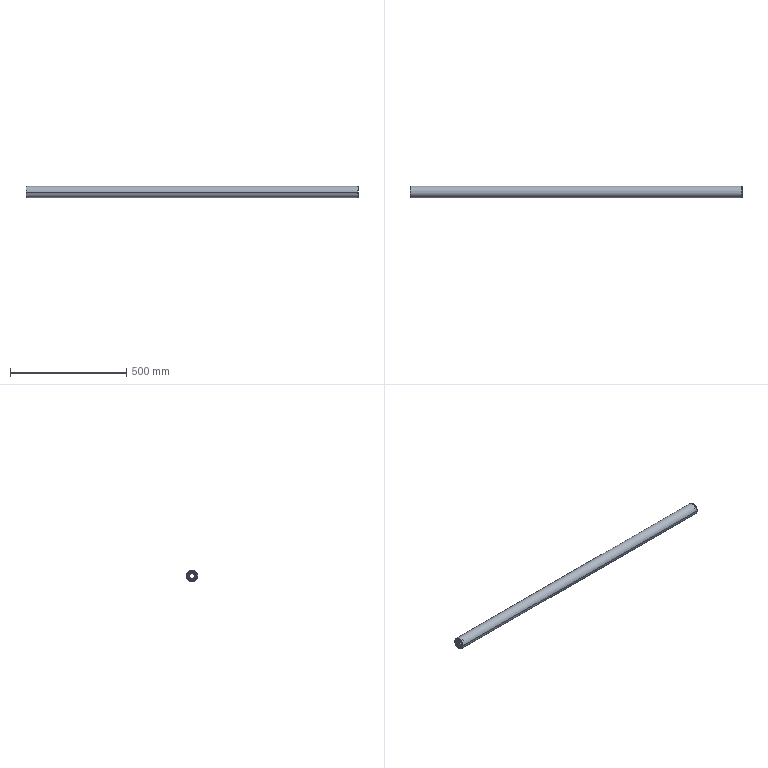Part | SolidWorks | features BaseBody 21 | 21 solids | 306 faces | box 1429 x 50 x 50 mm | volume 1432811 mm3 | cylinder 118 | plane 64 | sphere 60 | torus 52 | cone 12 | commonest cylinder face diameters 29.9 x27 32.1 x27 42 x12 2.5 x8 27.333 x8 34.667 x8